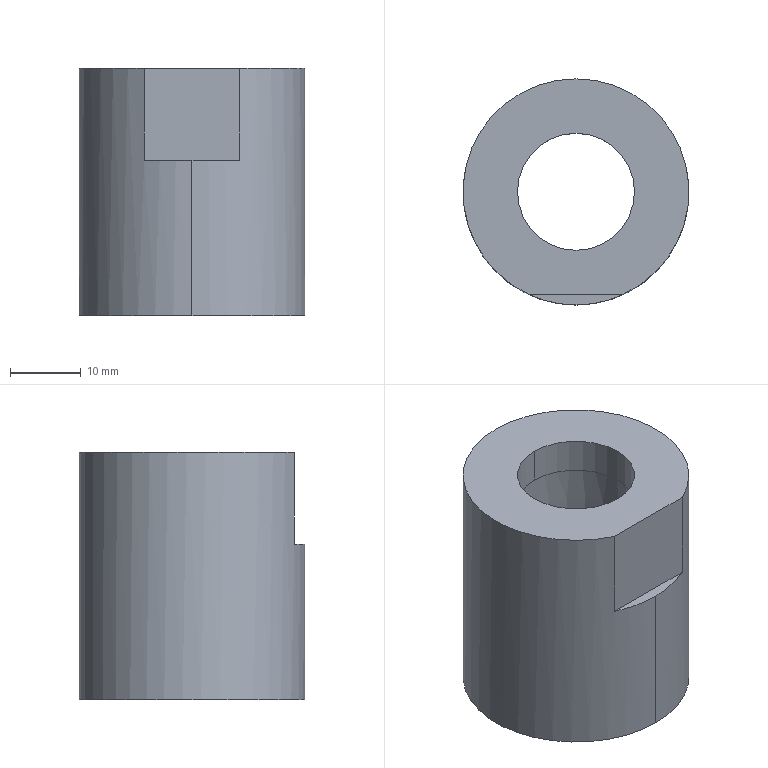Part | STEP file | 1_id4546_x_t | 1 solid | 9 faces | box 32 x 32 x 35 mm | volume 19791 mm3 | cylinder 4 | plane 4 | cone 1 | commonest cylinder face diameters 16.57 x2 32 x2
STEP:
#1=CARTESIAN_POINT('',(3203.,-147.215,-5.));
#2=VERTEX_POINT('',#1);
#3=CARTESIAN_POINT('',(3203.,-163.785,-5.));
#4=VERTEX_POINT('',#3);
#5=CARTESIAN_POINT('',(3203.,-155.5,-5.));
#6=DIRECTION('',(0.,0.,-1.));
#7=DIRECTION('',(-1.,0.,0.));
#8=AXIS2_PLACEMENT_3D('',#5,#6,#7);
#9=CIRCLE('',#8,8.285);
#10=EDGE_CURVE('',#2,#4,#9,.T.);
#11=ORIENTED_EDGE('',*,*,#10,.T.);
#12=CARTESIAN_POINT('',(3203.,-163.785,0.00001741));
#13=VERTEX_POINT('',#12);
#14=CARTESIAN_POINT('',(3203.,-163.785,-3.));
#15=DIRECTION('',(0.,0.,-1.));
#16=VECTOR('',#15,1.);
#17=LINE('',#14,#16);
#18=EDGE_CURVE('',#13,#4,#17,.T.);
#19=ORIENTED_EDGE('',*,*,#18,.F.);
#20=CARTESIAN_POINT('',(3203.,-147.215,0.00001741));
#21=VERTEX_POINT('',#20);
#22=CARTESIAN_POINT('',(3203.,-155.5,0.00001741));
#23=DIRECTION('',(0.,0.,-1.));
#24=DIRECTION('',(-1.,0.,0.));
#25=AXIS2_PLACEMENT_3D('',#22,#23,#24);
#26=CIRCLE('',#25,8.285);
#27=EDGE_CURVE('',#21,#13,#26,.T.);
#28=ORIENTED_EDGE('',*,*,#27,.F.);
#29=CARTESIAN_POINT('',(3203.,-147.215,-3.));
#30=DIRECTION('',(0.,0.,1.));
#31=VECTOR('',#30,1.);
#32=LINE('',#29,#31);
#33=EDGE_CURVE('',#2,#21,#32,.T.);
#34=ORIENTED_EDGE('',*,*,#33,.F.);
#35=EDGE_LOOP('',(#11,#19,#28,#34));
#36=FACE_OUTER_BOUND('',#35,.T.);
#37=CARTESIAN_POINT('',(3203.,-155.5,-3.));
#38=DIRECTION('',(0.,0.,-1.));
#39=DIRECTION('',(0.,1.,0.));
#40=AXIS2_PLACEMENT_3D('',#37,#38,#39);
#41=CYLINDRICAL_SURFACE('',#40,8.285);
#42=ADVANCED_FACE('',(#36),#41,.F.);
#43=CARTESIAN_POINT('',(3203.,-155.5,-5.));
#44=DIRECTION('',(0.,0.,-1.));
#45=DIRECTION('',(-1.,0.,0.));
#46=AXIS2_PLACEMENT_3D('',#43,#44,#45);
#47=CIRCLE('',#46,8.285);
#48=EDGE_CURVE('',#4,#2,#47,.T.);
#49=ORIENTED_EDGE('',*,*,#48,.T.);
#50=ORIENTED_EDGE('',*,*,#33,.T.);
#51=CARTESIAN_POINT('',(3203.,-155.5,0.00001741));
#52=DIRECTION('',(0.,0.,-1.));
#53=DIRECTION('',(-1.,0.,0.));
#54=AXIS2_PLACEMENT_3D('',#51,#52,#53);
#55=CIRCLE('',#54,8.285);
#56=EDGE_CURVE('',#13,#21,#55,.T.);
#57=ORIENTED_EDGE('',*,*,#56,.F.);
#58=ORIENTED_EDGE('',*,*,#18,.T.);
#59=EDGE_LOOP('',(#49,#50,#57,#58));
#60=FACE_OUTER_BOUND('',#59,.T.);
#61=CARTESIAN_POINT('',(3203.,-155.5,-3.));
#62=DIRECTION('',(0.,0.,-1.));
#63=DIRECTION('',(0.,1.,0.));
#64=AXIS2_PLACEMENT_3D('',#61,#62,#63);
#65=CYLINDRICAL_SURFACE('',#64,8.285);
#66=ADVANCED_FACE('',(#60),#65,.F.);
#67=CARTESIAN_POINT('',(3203.,-171.5,-35.));
#68=VERTEX_POINT('',#67);
#69=CARTESIAN_POINT('',(3203.,-139.5,-35.));
#70=VERTEX_POINT('',#69);
#71=CARTESIAN_POINT('',(3203.,-155.5,-35.));
#72=DIRECTION('',(0.,0.,1.));
#73=DIRECTION('',(-1.,0.,0.));
#74=AXIS2_PLACEMENT_3D('',#71,#72,#73);
#75=CIRCLE('',#74,16.);
#76=EDGE_CURVE('',#68,#70,#75,.T.);
#77=ORIENTED_EDGE('',*,*,#76,.F.);
#78=CARTESIAN_POINT('',(3203.,-155.5,-35.));
#79=DIRECTION('',(0.,0.,1.));
#80=DIRECTION('',(-1.,0.,0.));
#81=AXIS2_PLACEMENT_3D('',#78,#79,#80);
#82=CIRCLE('',#81,16.);
#83=EDGE_CURVE('',#70,#68,#82,.T.);
#84=ORIENTED_EDGE('',*,*,#83,.F.);
#85=EDGE_LOOP('',(#77,#84));
#86=FACE_BOUND('',#85,.T.);
#87=CARTESIAN_POINT('',(3193.929,-155.5,-35.));
#88=VERTEX_POINT('',#87);
#89=CARTESIAN_POINT('',(3203.,-155.5,-35.));
#90=DIRECTION('',(0.,0.,1.));
#91=DIRECTION('',(-1.,0.,0.));
#92=AXIS2_PLACEMENT_3D('',#89,#90,#91);
#93=CIRCLE('',#92,9.071);
#94=EDGE_CURVE('',#88,#88,#93,.T.);
#95=ORIENTED_EDGE('',*,*,#94,.T.);
#96=EDGE_LOOP('',(#95));
#97=FACE_BOUND('',#96,.T.);
#98=CARTESIAN_POINT('',(3203.,-161.75,-35.));
#99=DIRECTION('',(0.,0.,-1.));
#100=DIRECTION('',(0.,-1.,0.));
#101=AXIS2_PLACEMENT_3D('',#98,#99,#100);
#102=PLANE('',#101);
#103=ADVANCED_FACE('',(#86,#97),#102,.T.);
#104=CARTESIAN_POINT('',(3203.,-171.5,-13.));
#105=VERTEX_POINT('',#104);
#106=CARTESIAN_POINT('',(3203.,-171.5,-17.5));
#107=DIRECTION('',(0.,0.,1.));
#108=VECTOR('',#107,1.);
#109=LINE('',#106,#108);
#110=EDGE_CURVE('',#68,#105,#109,.T.);
#111=ORIENTED_EDGE('',*,*,#110,.F.);
#112=ORIENTED_EDGE('',*,*,#76,.T.);
#113=CARTESIAN_POINT('',(3203.,-139.5,0.00001741));
#114=VERTEX_POINT('',#113);
#115=CARTESIAN_POINT('',(3203.,-139.5,-17.5));
#116=DIRECTION('',(0.,0.,-1.));
#117=VECTOR('',#116,1.);
#118=LINE('',#115,#117);
#119=EDGE_CURVE('',#114,#70,#118,.T.);
#120=ORIENTED_EDGE('',*,*,#119,.F.);
#121=CARTESIAN_POINT('',(3209.764,-170.,0.00001741));
#122=VERTEX_POINT('',#121);
#123=CARTESIAN_POINT('',(3203.,-155.5,0.00001741));
#124=DIRECTION('',(0.,0.,1.));
#125=DIRECTION('',(-1.,0.,0.));
#126=AXIS2_PLACEMENT_3D('',#123,#124,#125);
#127=CIRCLE('',#126,16.);
#128=EDGE_CURVE('',#122,#114,#127,.T.);
#129=ORIENTED_EDGE('',*,*,#128,.F.);
#130=CARTESIAN_POINT('',(3209.764,-170.,-13.));
#131=VERTEX_POINT('',#130);
#132=CARTESIAN_POINT('',(3209.764,-170.,-17.5));
#133=DIRECTION('',(0.,0.,1.));
#134=VECTOR('',#133,1.);
#135=LINE('',#132,#134);
#136=EDGE_CURVE('',#131,#122,#135,.T.);
#137=ORIENTED_EDGE('',*,*,#136,.F.);
#138=CARTESIAN_POINT('',(3203.,-155.5,-13.));
#139=DIRECTION('',(0.,0.,1.));
#140=DIRECTION('',(-1.,0.,0.));
#141=AXIS2_PLACEMENT_3D('',#138,#139,#140);
#142=CIRCLE('',#141,16.);
#143=EDGE_CURVE('',#105,#131,#142,.T.);
#144=ORIENTED_EDGE('',*,*,#143,.F.);
#145=EDGE_LOOP('',(#111,#112,#120,#129,#137,#144));
#146=FACE_OUTER_BOUND('',#145,.T.);
#147=CARTESIAN_POINT('',(3203.,-155.5,-17.5));
#148=DIRECTION('',(0.,0.,1.));
#149=DIRECTION('',(0.,1.,0.));
#150=AXIS2_PLACEMENT_3D('',#147,#148,#149);
#151=CYLINDRICAL_SURFACE('',#150,16.);
#152=ADVANCED_FACE('',(#146),#151,.T.);
#153=ORIENTED_EDGE('',*,*,#119,.T.);
#154=ORIENTED_EDGE('',*,*,#83,.T.);
#155=ORIENTED_EDGE('',*,*,#110,.T.);
#156=CARTESIAN_POINT('',(3196.236,-170.,-13.));
#157=VERTEX_POINT('',#156);
#158=CARTESIAN_POINT('',(3203.,-155.5,-13.));
#159=DIRECTION('',(0.,0.,1.));
#160=DIRECTION('',(-1.,0.,0.));
#161=AXIS2_PLACEMENT_3D('',#158,#159,#160);
#162=CIRCLE('',#161,16.);
#163=EDGE_CURVE('',#157,#105,#162,.T.);
#164=ORIENTED_EDGE('',*,*,#163,.F.);
#165=CARTESIAN_POINT('',(3196.236,-170.,0.00001741));
#166=VERTEX_POINT('',#165);
#167=CARTESIAN_POINT('',(3196.236,-170.,-17.5));
#168=DIRECTION('',(0.,0.,-1.));
#169=VECTOR('',#168,1.);
#170=LINE('',#167,#169);
#171=EDGE_CURVE('',#166,#157,#170,.T.);
#172=ORIENTED_EDGE('',*,*,#171,.F.);
#173=CARTESIAN_POINT('',(3203.,-155.5,0.00001741));
#174=DIRECTION('',(0.,0.,1.));
#175=DIRECTION('',(-1.,0.,0.));
#176=AXIS2_PLACEMENT_3D('',#173,#174,#175);
#177=CIRCLE('',#176,16.);
#178=EDGE_CURVE('',#114,#166,#177,.T.);
#179=ORIENTED_EDGE('',*,*,#178,.F.);
#180=EDGE_LOOP('',(#153,#154,#155,#164,#172,#179));
#181=FACE_OUTER_BOUND('',#180,.T.);
#182=CARTESIAN_POINT('',(3203.,-155.5,-17.5));
#183=DIRECTION('',(0.,0.,1.));
#184=DIRECTION('',(0.,1.,0.));
#185=AXIS2_PLACEMENT_3D('',#182,#183,#184);
#186=CYLINDRICAL_SURFACE('',#185,16.);
#187=ADVANCED_FACE('',(#181),#186,.T.);
#188=CARTESIAN_POINT('',(3203.,-170.,0.00001741));
#189=DIRECTION('',(-1.,0.,0.));
#190=VECTOR('',#189,1.);
#191=LINE('',#188,#190);
#192=EDGE_CURVE('',#122,#166,#191,.T.);
#193=ORIENTED_EDGE('',*,*,#192,.F.);
#194=ORIENTED_EDGE('',*,*,#128,.T.);
#195=ORIENTED_EDGE('',*,*,#178,.T.);
#196=EDGE_LOOP('',(#193,#194,#195));
#197=FACE_BOUND('',#196,.T.);
#198=ORIENTED_EDGE('',*,*,#27,.T.);
#199=ORIENTED_EDGE('',*,*,#56,.T.);
#200=EDGE_LOOP('',(#198,#199));
#201=FACE_BOUND('',#200,.T.);
#202=CARTESIAN_POINT('',(3203.,-161.75,0.00001741));
#203=DIRECTION('',(0.,0.,1.));
#204=DIRECTION('',(0.,1.,0.));
#205=AXIS2_PLACEMENT_3D('',#202,#203,#204);
#206=PLANE('',#205);
#207=ADVANCED_FACE('',(#197,#201),#206,.T.);
#208=ORIENTED_EDGE('',*,*,#143,.T.);
#209=CARTESIAN_POINT('',(3203.,-170.,-13.));
#210=DIRECTION('',(1.,0.,0.));
#211=VECTOR('',#210,1.);
#212=LINE('',#209,#211);
#213=EDGE_CURVE('',#157,#131,#212,.T.);
#214=ORIENTED_EDGE('',*,*,#213,.F.);
#215=ORIENTED_EDGE('',*,*,#163,.T.);
#216=EDGE_LOOP('',(#208,#214,#215));
#217=FACE_OUTER_BOUND('',#216,.T.);
#218=CARTESIAN_POINT('',(3203.,-178.,-13.));
#219=DIRECTION('',(0.,0.,-1.));
#220=DIRECTION('',(0.,1.,0.));
#221=AXIS2_PLACEMENT_3D('',#218,#219,#220);
#222=PLANE('',#221);
#223=ADVANCED_FACE('',(#217),#222,.F.);
#224=ORIENTED_EDGE('',*,*,#136,.T.);
#225=ORIENTED_EDGE('',*,*,#192,.T.);
#226=ORIENTED_EDGE('',*,*,#171,.T.);
#227=ORIENTED_EDGE('',*,*,#213,.T.);
#228=EDGE_LOOP('',(#224,#225,#226,#227));
#229=FACE_OUTER_BOUND('',#228,.T.);
#230=CARTESIAN_POINT('',(3203.,-170.,-1.));
#231=DIRECTION('',(0.,1.,0.));
#232=DIRECTION('',(0.,0.,1.));
#233=AXIS2_PLACEMENT_3D('',#230,#231,#232);
#234=PLANE('',#233);
#235=ADVANCED_FACE('',(#229),#234,.F.);
#236=ORIENTED_EDGE('',*,*,#94,.F.);
#237=EDGE_LOOP('',(#236));
#238=FACE_BOUND('',#237,.T.);
#239=ORIENTED_EDGE('',*,*,#10,.F.);
#240=ORIENTED_EDGE('',*,*,#48,.F.);
#241=EDGE_LOOP('',(#239,#240));
#242=FACE_BOUND('',#241,.T.);
#243=CARTESIAN_POINT('',(3203.,-155.5,-5.));
#244=DIRECTION('',(0.,0.,-1.));
#245=DIRECTION('',(-1.,0.,0.));
#246=AXIS2_PLACEMENT_3D('',#243,#244,#245);
#247=CONICAL_SURFACE('',#246,8.285,1.5);
#248=ADVANCED_FACE('',(#238,#242),#247,.F.);
#249=CLOSED_SHELL('',(#42,#66,#103,#152,#187,#207,#223,#235,#248));
#250=MANIFOLD_SOLID_BREP('',#249);
#251=(LENGTH_UNIT()NAMED_UNIT(*)SI_UNIT(.MILLI.,.METRE.));
#252=UNCERTAINTY_MEASURE_WITH_UNIT(LENGTH_MEASURE(0.00002),#251,'','');
#253=(NAMED_UNIT(*)PLANE_ANGLE_UNIT()SI_UNIT($,.RADIAN.));
#254=PLANE_ANGLE_MEASURE_WITH_UNIT(PLANE_ANGLE_MEASURE(0.01745),#253);
#255=DIMENSIONAL_EXPONENTS(0.,0.,0.,0.,0.,0.,0.);
#256=(CONVERSION_BASED_UNIT('DEGREE',#254)NAMED_UNIT(#255)PLANE_ANGLE_UNIT());
#257=(NAMED_UNIT(*)SI_UNIT($,.STERADIAN.)SOLID_ANGLE_UNIT());
#258=(GEOMETRIC_REPRESENTATION_CONTEXT(3)GLOBAL_UNCERTAINTY_ASSIGNED_CONTEXT((#252))GLOBAL_UNIT_ASSIGNED_CONTEXT((#251,#256,#257))REPRESENTATION_CONTEXT('',''));
#259=ADVANCED_BREP_SHAPE_REPRESENTATION('',(#250),#258);